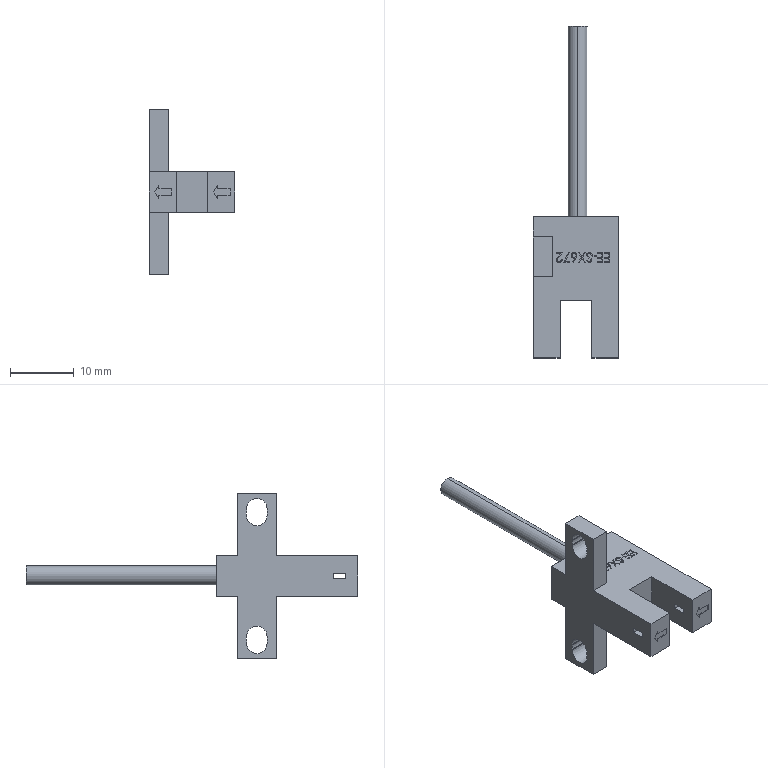Part | SolidWorks | features BaseBody 1 | 1 solid | 159 faces | box 13.4 x 52.2 x 26 mm | volume 2085 mm3 | plane 117 | spline 30 | cylinder 12 | commonest cylinder face diameters 3.2 x6 3.3 x4 3 x2